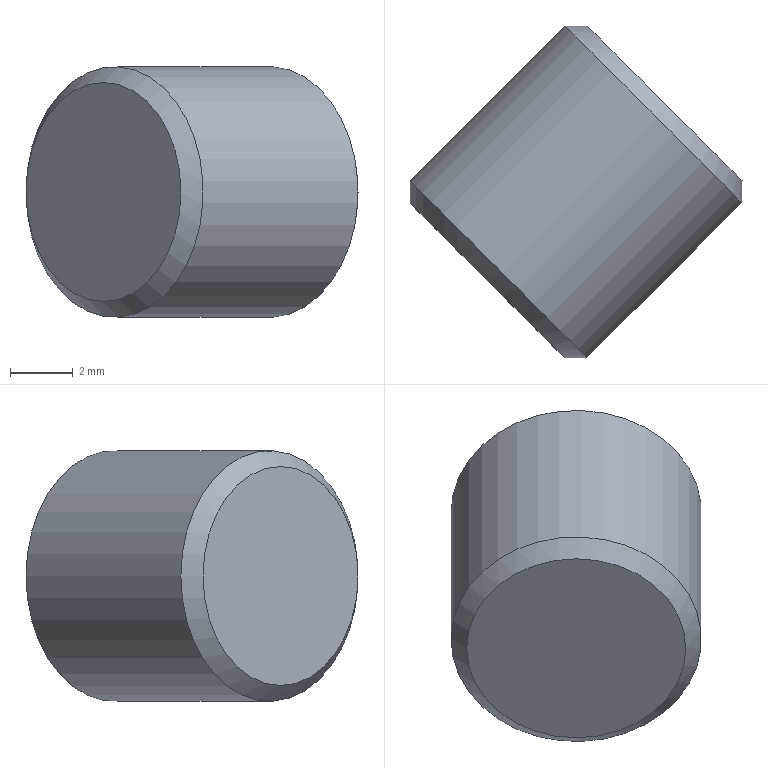Part | STEP file | gslz 2016.10.28-13_id654_x_t | 1 solid | 5 faces | box 10.607 x 10.607 x 8 mm | volume 396.102 mm3 | plane 2 | cone 2 | cylinder 1 | commonest cylinder face diameters 8 x1
STEP:
#1=CARTESIAN_POINT('',(0.,0.,0.));
#2=DIRECTION('',(0.,0.,1.));
#3=DIRECTION('',(1.,0.,0.));
#4=AXIS2_PLACEMENT_3D('',#1,#2,#3);
#5=CARTESIAN_POINT('',(578.137,188.016,-21.226));
#6=VERTEX_POINT('',#5);
#7=CARTESIAN_POINT('',(580.965,185.188,-21.226));
#8=DIRECTION('',(0.7071,0.7071,0.));
#9=DIRECTION('',(-0.7071,0.7071,0.));
#10=AXIS2_PLACEMENT_3D('',#7,#8,#9);
#11=CIRCLE('',#10,4.);
#12=CARTESIAN_POINT('',(579.198,183.42,-21.226));
#13=DIRECTION('',(0.7071,0.7071,0.));
#14=DIRECTION('',(-0.7071,0.7071,0.));
#15=AXIS2_PLACEMENT_3D('',#12,#13,#14);
#16=CYLINDRICAL_SURFACE('',#15,4.);
#17=CARTESIAN_POINT('',(0.,2.5));
#18=DIRECTION('',(1.,0.));
#19=VECTOR('',#18,1.);
#20=LINE('',#17,#19);
#21=(GEOMETRIC_REPRESENTATION_CONTEXT(2)PARAMETRIC_REPRESENTATION_CONTEXT()REPRESENTATION_CONTEXT('',''));
#22=DEFINITIONAL_REPRESENTATION('',(#20),#21);
#23=PCURVE('',#16,#22);
#24=CARTESIAN_POINT('',(580.965,185.188,-21.226));
#25=DIRECTION('',(0.7071,0.7071,0.));
#26=DIRECTION('',(-0.7071,0.7071,0.));
#27=AXIS2_PLACEMENT_3D('',#24,#25,#26);
#28=CONICAL_SURFACE('',#27,4.,0.7854);
#29=CARTESIAN_POINT('',(0.,0.));
#30=DIRECTION('',(1.,0.));
#31=VECTOR('',#30,1.);
#32=LINE('',#29,#31);
#33=(GEOMETRIC_REPRESENTATION_CONTEXT(2)PARAMETRIC_REPRESENTATION_CONTEXT()REPRESENTATION_CONTEXT('',''));
#34=DEFINITIONAL_REPRESENTATION('',(#32),#33);
#35=PCURVE('',#28,#34);
#36=SURFACE_CURVE('',#11,(#23,#35),.PCURVE_S1.);
#37=EDGE_CURVE('',#6,#6,#36,.T.);
#38=ORIENTED_EDGE('',*,*,#37,.T.);
#39=CARTESIAN_POINT('',(583.087,192.966,-21.226));
#40=VERTEX_POINT('',#39);
#41=CARTESIAN_POINT('',(578.137,188.016,-21.226));
#42=CARTESIAN_POINT('',(583.087,192.966,-21.226));
#43=B_SPLINE_CURVE_WITH_KNOTS('',1,(#41,#42),.UNSPECIFIED.,.F.,.F.,(2,2),(2.5,9.5),.PIECEWISE_BEZIER_KNOTS.);
#44=CARTESIAN_POINT('',(6.283,0.));
#45=DIRECTION('',(0.,1.));
#46=VECTOR('',#45,1.);
#47=LINE('',#44,#46);
#48=(GEOMETRIC_REPRESENTATION_CONTEXT(2)PARAMETRIC_REPRESENTATION_CONTEXT()REPRESENTATION_CONTEXT('',''));
#49=DEFINITIONAL_REPRESENTATION('',(#47),#48);
#50=PCURVE('',#16,#49);
#51=CARTESIAN_POINT('',(0.,0.));
#52=DIRECTION('',(0.,1.));
#53=VECTOR('',#52,1.);
#54=LINE('',#51,#53);
#55=(GEOMETRIC_REPRESENTATION_CONTEXT(2)PARAMETRIC_REPRESENTATION_CONTEXT()REPRESENTATION_CONTEXT('',''));
#56=DEFINITIONAL_REPRESENTATION('',(#54),#55);
#57=PCURVE('',#16,#56);
#58=SEAM_CURVE('',#43,(#50,#57),.PCURVE_S1.);
#59=EDGE_CURVE('',#6,#40,#58,.T.);
#60=ORIENTED_EDGE('',*,*,#59,.T.);
#61=CARTESIAN_POINT('',(585.915,190.138,-21.226));
#62=DIRECTION('',(-0.7071,-0.7071,0.));
#63=DIRECTION('',(-0.7071,0.7071,0.));
#64=AXIS2_PLACEMENT_3D('',#61,#62,#63);
#65=CIRCLE('',#64,4.);
#66=CARTESIAN_POINT('',(6.283,9.5));
#67=DIRECTION('',(-1.,0.));
#68=VECTOR('',#67,1.);
#69=LINE('',#66,#68);
#70=(GEOMETRIC_REPRESENTATION_CONTEXT(2)PARAMETRIC_REPRESENTATION_CONTEXT()REPRESENTATION_CONTEXT('',''));
#71=DEFINITIONAL_REPRESENTATION('',(#69),#70);
#72=PCURVE('',#16,#71);
#73=CARTESIAN_POINT('',(586.269,190.491,-21.226));
#74=DIRECTION('',(-0.7071,-0.7071,0.));
#75=DIRECTION('',(0.7071,-0.7071,0.));
#76=AXIS2_PLACEMENT_3D('',#73,#74,#75);
#77=CONICAL_SURFACE('',#76,3.5,0.7854);
#78=CARTESIAN_POINT('',(3.142,0.5));
#79=DIRECTION('',(1.,0.));
#80=VECTOR('',#79,1.);
#81=LINE('',#78,#80);
#82=(GEOMETRIC_REPRESENTATION_CONTEXT(2)PARAMETRIC_REPRESENTATION_CONTEXT()REPRESENTATION_CONTEXT('',''));
#83=DEFINITIONAL_REPRESENTATION('',(#81),#82);
#84=PCURVE('',#77,#83);
#85=SURFACE_CURVE('',#65,(#72,#84),.PCURVE_S1.);
#86=EDGE_CURVE('',#40,#40,#85,.T.);
#87=ORIENTED_EDGE('',*,*,#86,.T.);
#88=ORIENTED_EDGE('',*,*,#59,.F.);
#89=EDGE_LOOP('',(#38,#60,#87,#88));
#90=FACE_BOUND('',#89,.T.);
#91=ADVANCED_FACE('',(#90),#16,.T.);
#92=CARTESIAN_POINT('',(578.137,187.309,-21.226));
#93=VERTEX_POINT('',#92);
#94=CARTESIAN_POINT('',(580.612,184.834,-21.226));
#95=DIRECTION('',(-0.7071,-0.7071,0.));
#96=DIRECTION('',(-0.7071,0.7071,0.));
#97=AXIS2_PLACEMENT_3D('',#94,#95,#96);
#98=CIRCLE('',#97,3.5);
#99=CARTESIAN_POINT('',(580.612,184.834,-21.226));
#100=DIRECTION('',(0.7071,0.7071,0.));
#101=DIRECTION('',(-0.7071,0.7071,0.));
#102=AXIS2_PLACEMENT_3D('',#99,#100,#101);
#103=PLANE('',#102);
#104=CARTESIAN_POINT('',(3.5,0.));
#105=CARTESIAN_POINT('',(3.5,-6.062));
#106=CARTESIAN_POINT('',(-1.75,-3.031));
#107=CARTESIAN_POINT('',(-7.,0.));
#108=CARTESIAN_POINT('',(-1.75,3.031));
#109=CARTESIAN_POINT('',(3.5,6.062));
#110=CARTESIAN_POINT('',(3.5,0.));
#111=(BOUNDED_CURVE()B_SPLINE_CURVE(2,(#104,#105,#106,#107,#108,#109,#110),.UNSPECIFIED.,.T.,.F.)B_SPLINE_CURVE_WITH_KNOTS((1,2,2,2,2,1),(-2.094,0.,2.094,4.189,6.283,8.378),.UNSPECIFIED.)CURVE()GEOMETRIC_REPRESENTATION_ITEM()RATIONAL_B_SPLINE_CURVE((1.,0.5,1.,0.5,1.,0.5,1.))REPRESENTATION_ITEM(''));
#112=(GEOMETRIC_REPRESENTATION_CONTEXT(2)PARAMETRIC_REPRESENTATION_CONTEXT()REPRESENTATION_CONTEXT('',''));
#113=DEFINITIONAL_REPRESENTATION('',(#111),#112);
#114=PCURVE('',#103,#113);
#115=CARTESIAN_POINT('',(6.283,-0.5));
#116=DIRECTION('',(-1.,0.));
#117=VECTOR('',#116,1.);
#118=LINE('',#115,#117);
#119=(GEOMETRIC_REPRESENTATION_CONTEXT(2)PARAMETRIC_REPRESENTATION_CONTEXT()REPRESENTATION_CONTEXT('',''));
#120=DEFINITIONAL_REPRESENTATION('',(#118),#119);
#121=PCURVE('',#28,#120);
#122=SURFACE_CURVE('',#98,(#114,#121),.PCURVE_S1.);
#123=EDGE_CURVE('',#93,#93,#122,.T.);
#124=ORIENTED_EDGE('',*,*,#123,.T.);
#125=EDGE_LOOP('',(#124));
#126=FACE_BOUND('',#125,.T.);
#127=ADVANCED_FACE('',(#126),#103,.F.);
#128=CARTESIAN_POINT('',(583.794,192.966,-21.226));
#129=VERTEX_POINT('',#128);
#130=CARTESIAN_POINT('',(586.269,190.491,-21.226));
#131=DIRECTION('',(0.7071,0.7071,0.));
#132=DIRECTION('',(-0.7071,0.7071,0.));
#133=AXIS2_PLACEMENT_3D('',#130,#131,#132);
#134=CIRCLE('',#133,3.5);
#135=CARTESIAN_POINT('',(586.269,190.491,-21.226));
#136=DIRECTION('',(0.7071,0.7071,0.));
#137=DIRECTION('',(-0.7071,0.7071,0.));
#138=AXIS2_PLACEMENT_3D('',#135,#136,#137);
#139=PLANE('',#138);
#140=CARTESIAN_POINT('',(0.,0.));
#141=DIRECTION('',(1.,0.));
#142=AXIS2_PLACEMENT_2D('',#140,#141);
#143=CIRCLE('',#142,3.5);
#144=(GEOMETRIC_REPRESENTATION_CONTEXT(2)PARAMETRIC_REPRESENTATION_CONTEXT()REPRESENTATION_CONTEXT('',''));
#145=DEFINITIONAL_REPRESENTATION('',(#143),#144);
#146=PCURVE('',#139,#145);
#147=CARTESIAN_POINT('',(9.425,0.));
#148=DIRECTION('',(-1.,0.));
#149=VECTOR('',#148,1.);
#150=LINE('',#147,#149);
#151=(GEOMETRIC_REPRESENTATION_CONTEXT(2)PARAMETRIC_REPRESENTATION_CONTEXT()REPRESENTATION_CONTEXT('',''));
#152=DEFINITIONAL_REPRESENTATION('',(#150),#151);
#153=PCURVE('',#77,#152);
#154=SURFACE_CURVE('',#134,(#146,#153),.PCURVE_S1.);
#155=EDGE_CURVE('',#129,#129,#154,.T.);
#156=ORIENTED_EDGE('',*,*,#155,.T.);
#157=EDGE_LOOP('',(#156));
#158=FACE_BOUND('',#157,.T.);
#159=ADVANCED_FACE('',(#158),#139,.T.);
#160=ORIENTED_EDGE('',*,*,#86,.F.);
#161=CARTESIAN_POINT('',(583.794,192.966,-21.226));
#162=CARTESIAN_POINT('',(583.087,192.966,-21.226));
#163=B_SPLINE_CURVE_WITH_KNOTS('',1,(#161,#162),.UNSPECIFIED.,.F.,.F.,(2,2),(0.,0.7071),.PIECEWISE_BEZIER_KNOTS.);
#164=CARTESIAN_POINT('',(3.142,0.));
#165=DIRECTION('',(0.,1.));
#166=VECTOR('',#165,1.);
#167=LINE('',#164,#166);
#168=(GEOMETRIC_REPRESENTATION_CONTEXT(2)PARAMETRIC_REPRESENTATION_CONTEXT()REPRESENTATION_CONTEXT('',''));
#169=DEFINITIONAL_REPRESENTATION('',(#167),#168);
#170=PCURVE('',#77,#169);
#171=CARTESIAN_POINT('',(9.425,0.));
#172=DIRECTION('',(0.,1.));
#173=VECTOR('',#172,1.);
#174=LINE('',#171,#173);
#175=(GEOMETRIC_REPRESENTATION_CONTEXT(2)PARAMETRIC_REPRESENTATION_CONTEXT()REPRESENTATION_CONTEXT('',''));
#176=DEFINITIONAL_REPRESENTATION('',(#174),#175);
#177=PCURVE('',#77,#176);
#178=SEAM_CURVE('',#163,(#170,#177),.PCURVE_S1.);
#179=EDGE_CURVE('',#129,#40,#178,.T.);
#180=ORIENTED_EDGE('',*,*,#179,.F.);
#181=ORIENTED_EDGE('',*,*,#155,.F.);
#182=ORIENTED_EDGE('',*,*,#179,.T.);
#183=EDGE_LOOP('',(#160,#180,#181,#182));
#184=FACE_BOUND('',#183,.T.);
#185=ADVANCED_FACE('',(#184),#77,.T.);
#186=ORIENTED_EDGE('',*,*,#123,.F.);
#187=CARTESIAN_POINT('',(578.137,187.309,-21.226));
#188=CARTESIAN_POINT('',(578.137,188.016,-21.226));
#189=B_SPLINE_CURVE_WITH_KNOTS('',1,(#187,#188),.UNSPECIFIED.,.F.,.F.,(2,2),(-0.7071,0.),.PIECEWISE_BEZIER_KNOTS.);
#190=CARTESIAN_POINT('',(6.283,0.));
#191=DIRECTION('',(0.,1.));
#192=VECTOR('',#191,1.);
#193=LINE('',#190,#192);
#194=(GEOMETRIC_REPRESENTATION_CONTEXT(2)PARAMETRIC_REPRESENTATION_CONTEXT()REPRESENTATION_CONTEXT('',''));
#195=DEFINITIONAL_REPRESENTATION('',(#193),#194);
#196=PCURVE('',#28,#195);
#197=CARTESIAN_POINT('',(0.,0.));
#198=DIRECTION('',(0.,1.));
#199=VECTOR('',#198,1.);
#200=LINE('',#197,#199);
#201=(GEOMETRIC_REPRESENTATION_CONTEXT(2)PARAMETRIC_REPRESENTATION_CONTEXT()REPRESENTATION_CONTEXT('',''));
#202=DEFINITIONAL_REPRESENTATION('',(#200),#201);
#203=PCURVE('',#28,#202);
#204=SEAM_CURVE('',#189,(#196,#203),.PCURVE_S1.);
#205=EDGE_CURVE('',#93,#6,#204,.T.);
#206=ORIENTED_EDGE('',*,*,#205,.T.);
#207=ORIENTED_EDGE('',*,*,#37,.F.);
#208=ORIENTED_EDGE('',*,*,#205,.F.);
#209=EDGE_LOOP('',(#186,#206,#207,#208));
#210=FACE_BOUND('',#209,.T.);
#211=ADVANCED_FACE('',(#210),#28,.T.);
#212=CLOSED_SHELL('',(#91,#127,#159,#185,#211));
#213=MANIFOLD_SOLID_BREP('',#212);
#214=(LENGTH_UNIT()NAMED_UNIT(*)SI_UNIT(.MILLI.,.METRE.));
#215=UNCERTAINTY_MEASURE_WITH_UNIT(LENGTH_MEASURE(0.00001),#214,'','');
#216=(NAMED_UNIT(*)PLANE_ANGLE_UNIT()SI_UNIT($,.RADIAN.));
#217=(NAMED_UNIT(*)SI_UNIT($,.STERADIAN.)SOLID_ANGLE_UNIT());
#218=(GEOMETRIC_REPRESENTATION_CONTEXT(3)GLOBAL_UNCERTAINTY_ASSIGNED_CONTEXT((#215))GLOBAL_UNIT_ASSIGNED_CONTEXT((#214,#216,#217))REPRESENTATION_CONTEXT('',''));
#219=ADVANCED_BREP_SHAPE_REPRESENTATION('',(#4,#213),#218);